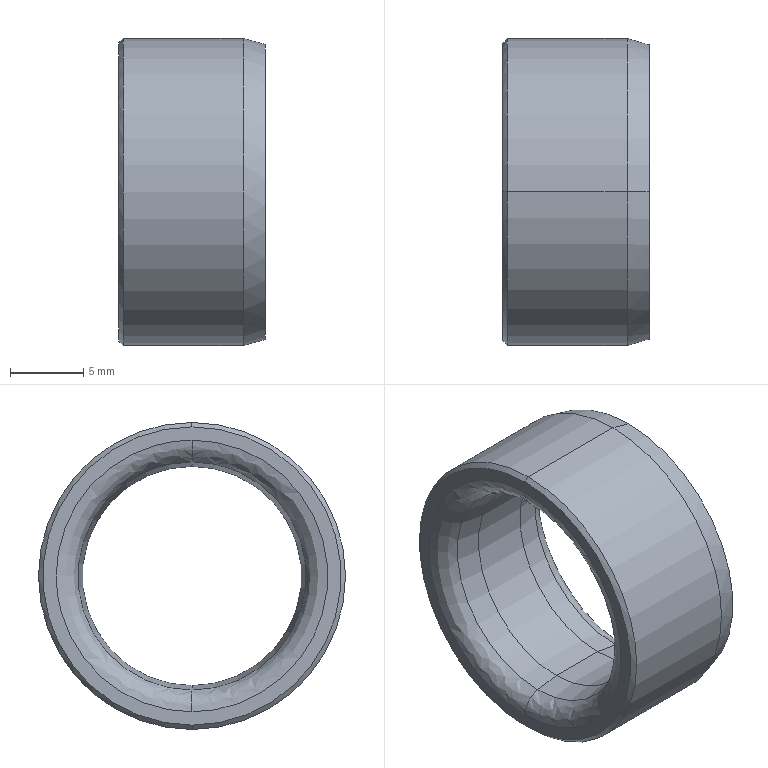Part | STEP file | 0217_004_MPBZ15-10 | 1 solid | 18 faces | box 10 x 21 x 21 mm | volume 1565 mm3 | cone 8 | spline 4 | cylinder 4 | plane 2 | commonest cylinder face diameters 15 x2 21 x2